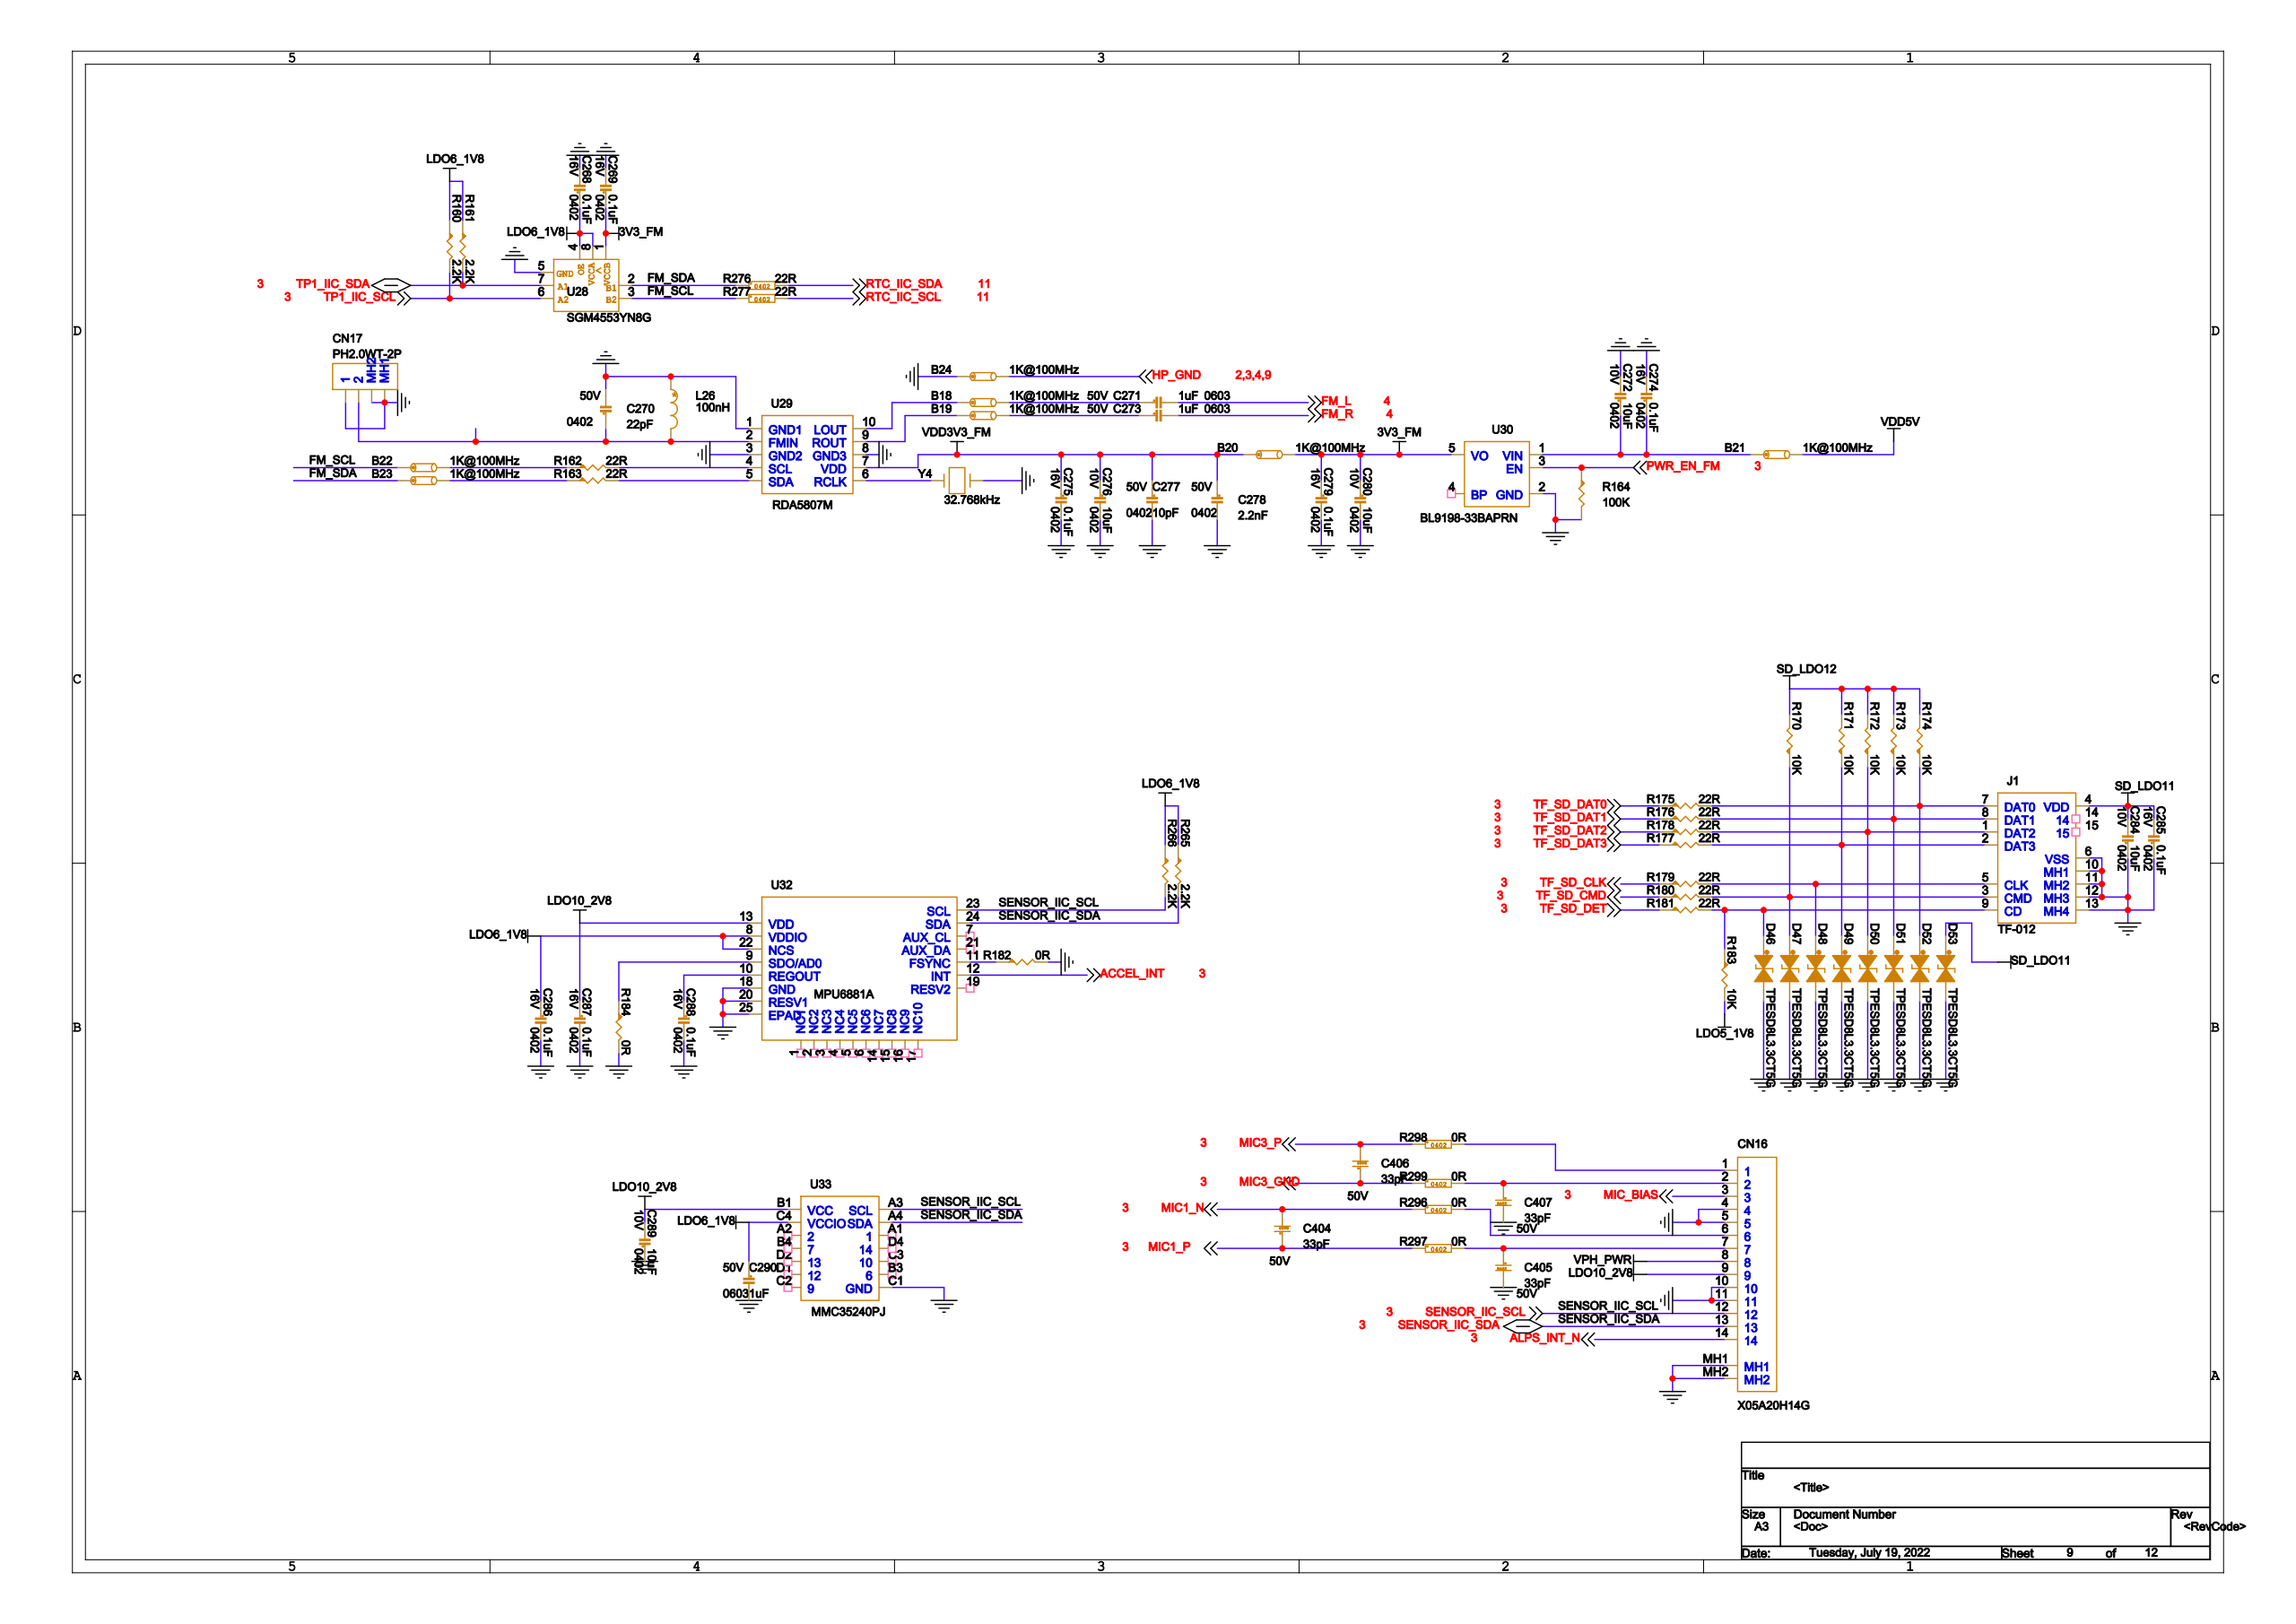Circuit board | Cadence Allegro | 970 parts | 627 nets | one sheet of the schematic
Parts on this sheet (reference | value | footprint):
B18 | 1K@100MHz | R0603
B19 | 1K@100MHz | R0603
B20 | 1K@100MHz | R0603
B21 | 1K@100MHz | R0603
B22 | 1K@100MHz | R0603
B23 | 1K@100MHz | R0603
B24 | 1K@100MHz | R0603
C268 | 0.1uF | C0402
C269 | 0.1uF | C0402
C270 | 22pF | C0402
C271 | 1uF | C0603
C272 | 10uF | C0402
C273 | 1uF | C0603
C274 | 0.1uF | C0402
C275 | 0.1uF | C0402
C276 | 10uF | C0402
C277 | 10pF | C0402
C278 | 2.2nF | C0402
C279 | 0.1uF | C0402
C280 | 10uF | C0402
C284 | 10uF | C0402
C285 | 0.1uF | C0402
C286 | 0.1uF | C0402
C287 | 0.1uF | C0402
C288 | 0.1uF | C0402
C289 | 10uF | C0402
C290 | 1uF | C0603
C404 | 33pF | C0402
C405 | 33pF | C0402
C406 | 33pF | C0402
C407 | 33pF | C0402
CN16 | X05A20H14G | FPC-14-0P5-2MMH
CN17 | PH2.0WT-2P | PH20_2_SMD_B
D46 | TPESD8L3.3CT5G | DFN1006_2L
D47 | TPESD8L3.3CT5G | DFN1006_2L
D48 | TPESD8L3.3CT5G | DFN1006_2L
D49 | TPESD8L3.3CT5G | DFN1006_2L
D50 | TPESD8L3.3CT5G | DFN1006_2L
D51 | TPESD8L3.3CT5G | DFN1006_2L
D52 | TPESD8L3.3CT5G | DFN1006_2L
D53 | TPESD8L3.3CT5G | DFN1006_2L
J1 | TF-012 | TFCARD1
L26 | 100nH | R0603
R160 | 2.2K | R0402
R161 | 2.2K | R0402
R162 | 22R | R0402
R163 | 22R | R0402
R164 | 100K | R0402
R170 | 10K | R0402
R171 | 10K | R0402
R172 | 10K | R0402
R173 | 10K | R0402
R174 | 10K | R0402
R175 | 22R | R0402
R176 | 22R | R0402
R177 | 22R | R0402
R178 | 22R | R0402
R179 | 22R | R0402
R180 | 22R | R0402
R181 | 22R | R0402
R182 | 0R | R0402
R183 | 10K | R0402
R184 | 0R | R0402
R265 | 2.2K | R0402
R266 | 2.2K | R0402
R276 | 22R | R0402
R277 | 22R | R0402
R296 | 0R | R0402
R297 | 0R | R0402
R298 | 0R | R0402
R299 | 0R | R0402
U28 | SGM4553YN8G | SOT23_8
U29 | RDA5807M | MSOP10
U30 | BL9198-33BAPRN | SOT23-5
U32 | MPU6881A | QFN24_0P4_3X3
U33 | MMC35240PJ | MMC35240
Y4 | 32.768kHz | X3215
Nets of these parts (net: part-pin ...):
VDD5V: B21-2
GND: B24-1 C268-2 C269-2 C270-2 C272-2 C274-2 C275-2 C276-2 C277-2 C278-2 C279-2 C280-2 C284-1 C285-1 C286-2 C287-2 C288-2 C289-1 C290-2 C405-2 C407-2 CN16-4 CN16-5 CN16-10 CN16-11 CN16-MH1 CN16-MH2 CN17-1 CN17-MH1 CN17-MH2 D46-1 D47-1 D48-1 D49-1 D50-1 D51-1 D52-1 D53-1 J1-6 J1-10 J1-11 J1-12 J1-13 L26-1 R164-2 R182-2 R184-2 U28-5 U29-1 U29-3 U29-8 U30-2 U32-18 U32-20 U32-25 U33-C1 Y4-2
LDO6_1V8: C268-1 C286-1 C290-1 R160-1 R161-1 R265-1 R266-1 U28-4 U28-8 U32-8 U32-22 U33-C4
MIC1_P: C404-1 R297-1
MIC1_N: C404-2 R296-1
N19539673: C405-1 CN16-7 R297-2
MIC3_GND: C406-1 R299-1
MIC3_P: C406-2 R298-1
N19698796: C407-1 CN16-2 R299-2
SENSOR_IIC_SCL: CN16-12 R266-2 U32-23 U33-A3
SENSOR_IIC_SDA: CN16-13 R265-2 U32-24 U33-A4
LDO10_2V8: C287-1 C289-2 CN16-9 U32-13 U33-B1
N19539572: CN16-6 R296-2
N19698794: CN16-1 R298-2
LDO5_1V8: R183-2
FM_SDA: B23-1 R276-1 U28-2
RTC_IIC_SDA: R276-2
FM_SCL: B22-1 R277-1 U28-3
RTC_IIC_SCL: R277-2
N19309335: C270-1 CN17-2 L26-2 U29-2
ALPS_INT_N: CN16-14
MIC_BIAS: CN16-3
VPH_PWR: CN16-8
HP_GND: B24-2
N19310124: B18-1 U29-10
N19310133: B18-2 C271-1
N19310115: B19-1 U29-9
N19310136: B19-2 C273-1
VDD3V3_FM: B20-1 C275-1 C276-1 C277-1 C278-1 U29-7
3V3_FM: B20-2 C269-1 C279-1 C280-1 U28-1 U30-5
N19310847: B21-1 C272-1 C274-1 U30-1
N19309442: B22-2 R162-1
N19309445: B23-2 R163-1
FM_L: C271-2
FM_R: C273-2
N19377839: D46-2 J1-9 R181-2 R183-1
N19378998: D47-2 J1-3 R170-1 R180-2
N19379001: D48-2 J1-5 R179-2
N19379018: D49-2 J1-2 R171-1 R177-2
N19379028: D50-2 J1-1 R172-1 R178-2
N19379038: D51-2 J1-8 R173-1 R176-2
N19379041: D52-2 J1-7 R174-1 R175-2
SD_LDO11: C284-2 C285-2 D53-2 J1-4
N19313915: R182-1 U32-11
N19313352: R184-1 U32-9
PWR_EN_FM: R164-1 U30-3
N19309451: R162-2 U29-4
N19309448: R163-2 U29-5
TF_SD_DAT0: R175-1
TF_SD_DAT1: R176-1
TF_SD_DAT2: R178-1
TF_SD_DAT3: R177-1
TF_SD_CLK: R179-1
TF_SD_CMD: R180-1
TF_SD_DET: R181-1
SD_LDO12: R170-2 R171-2 R172-2 R173-2 R174-2
TP1_IIC_SCL: R160-2 U28-6
TP1_IIC_SDA: R161-2 U28-7
N19309513: U29-6 Y4-1
ACCEL_INT: U32-12
N19313158: C288-1 U32-10